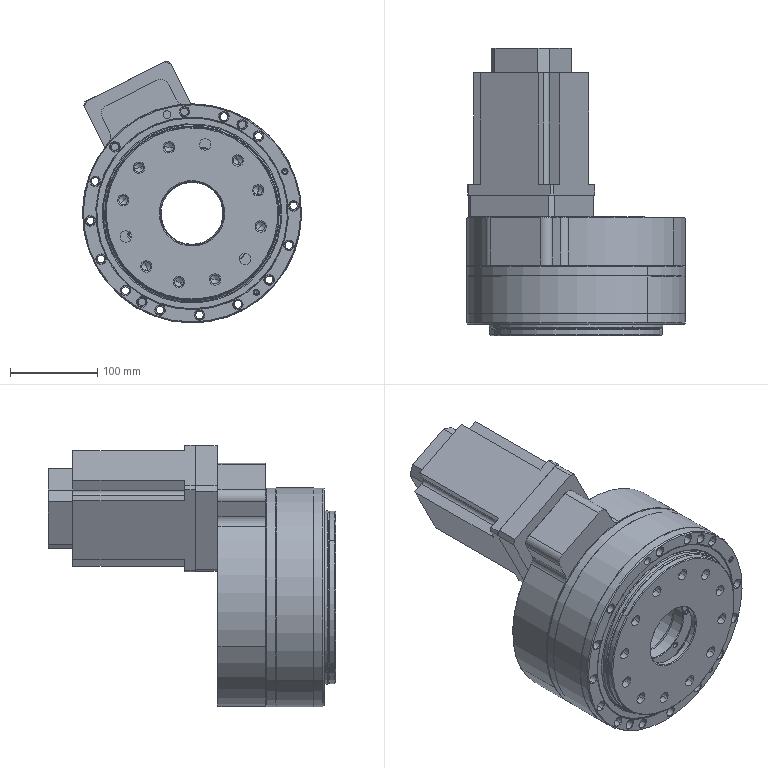Part | SolidWorks | 8 solids | 925 faces | box 250.5 x 328.6 x 299.355 mm | volume 6826026 mm3 | cylinder 425 | cone 279 | plane 197 | torus 24 | commonest cylinder face diameters 12.6 x40 11 x34 8.5 x32 13 x24 15 x20 9 x18